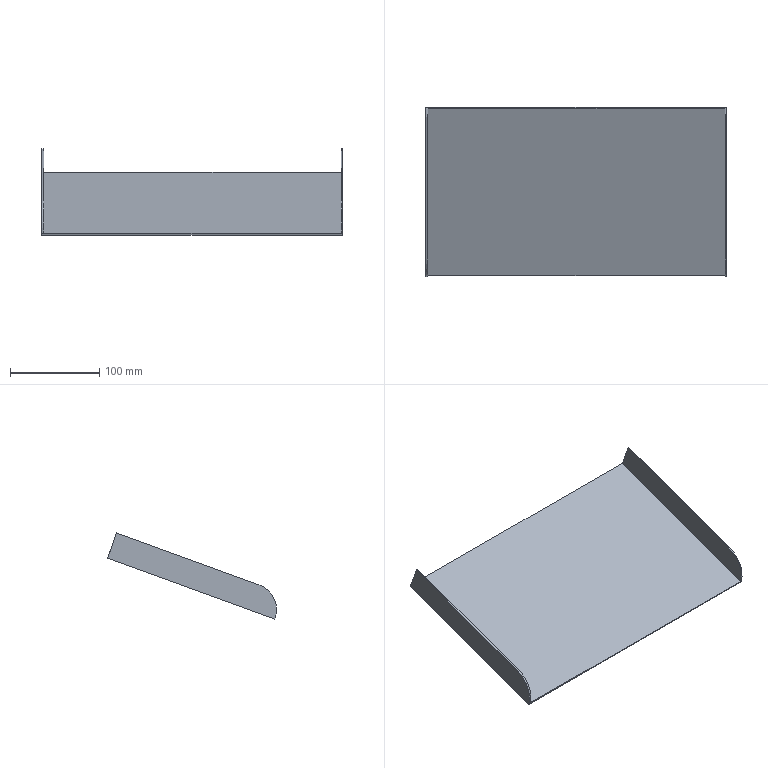Part | NX | features solid 2 | 1 solid | 12 faces | box 337.136 x 189.748 x 96.595 mm | volume 151075 mm3 | plane 10 | cylinder 2 | commonest cylinder face diameters 60 x2
STEP:
#1=CARTESIAN_POINT('',(-937.864,-997.876,-367.964));
#2=VERTEX_POINT('',#1);
#3=CARTESIAN_POINT('',(-938.864,-997.876,-367.964));
#4=VERTEX_POINT('',#3);
#5=CARTESIAN_POINT('',(-937.864,-997.876,-367.964));
#6=DIRECTION('',(1.,0.,0.));
#7=VECTOR('',#6,1000.);
#8=LINE('',#5,#7);
#9=EDGE_CURVE('',#2,#4,#8,.F.);
#10=ORIENTED_EDGE('',*,*,#9,.T.);
#11=CARTESIAN_POINT('',(-938.864,-810.,-299.582));
#12=VERTEX_POINT('',#11);
#13=CARTESIAN_POINT('',(-938.864,-838.191,-309.843));
#14=DIRECTION('',(0.,0.9397,0.342));
#15=VECTOR('',#14,1000.);
#16=LINE('',#13,#15);
#17=EDGE_CURVE('',#4,#12,#16,.T.);
#18=ORIENTED_EDGE('',*,*,#17,.T.);
#19=CARTESIAN_POINT('',(-1273.,-810.,-299.582));
#20=VERTEX_POINT('',#19);
#21=CARTESIAN_POINT('',(-1268.,-810.,-299.582));
#22=DIRECTION('',(-1.,0.,0.));
#23=VECTOR('',#22,1000.);
#24=LINE('',#21,#23);
#25=EDGE_CURVE('',#20,#12,#24,.F.);
#26=ORIENTED_EDGE('',*,*,#25,.F.);
#27=CARTESIAN_POINT('',(-1273.,-997.876,-367.964));
#28=VERTEX_POINT('',#27);
#29=CARTESIAN_POINT('',(-1273.,-838.191,-309.843));
#30=DIRECTION('',(0.,0.9397,0.342));
#31=VECTOR('',#30,1000.);
#32=LINE('',#29,#31);
#33=EDGE_CURVE('',#28,#20,#32,.T.);
#34=ORIENTED_EDGE('',*,*,#33,.F.);
#35=CARTESIAN_POINT('',(-1275.,-997.876,-367.964));
#36=VERTEX_POINT('',#35);
#37=CARTESIAN_POINT('',(-1280.,-997.876,-367.964));
#38=DIRECTION('',(-1.,0.,0.));
#39=VECTOR('',#38,1000.);
#40=LINE('',#37,#39);
#41=EDGE_CURVE('',#28,#36,#40,.T.);
#42=ORIENTED_EDGE('',*,*,#41,.T.);
#43=CARTESIAN_POINT('',(-1275.,-997.939,-367.986));
#44=VERTEX_POINT('',#43);
#45=CARTESIAN_POINT('',(-1275.,-838.191,-309.843));
#46=DIRECTION('',(0.,-0.9397,-0.342));
#47=VECTOR('',#46,1000.);
#48=LINE('',#45,#47);
#49=EDGE_CURVE('',#36,#44,#48,.T.);
#50=ORIENTED_EDGE('',*,*,#49,.T.);
#51=CARTESIAN_POINT('',(-937.864,-997.939,-367.986));
#52=VERTEX_POINT('',#51);
#53=CARTESIAN_POINT('',(-1268.,-997.939,-367.986));
#54=DIRECTION('',(1.,0.,0.));
#55=VECTOR('',#54,1000.);
#56=LINE('',#53,#55);
#57=EDGE_CURVE('',#44,#52,#56,.T.);
#58=ORIENTED_EDGE('',*,*,#57,.T.);
#59=CARTESIAN_POINT('',(-937.864,-838.191,-309.843));
#60=DIRECTION('',(0.,0.9397,0.342));
#61=VECTOR('',#60,1000.);
#62=LINE('',#59,#61);
#63=EDGE_CURVE('',#2,#52,#62,.F.);
#64=ORIENTED_EDGE('',*,*,#63,.F.);
#65=EDGE_LOOP('',(#10,#18,#26,#34,#42,#50,#58,#64));
#66=FACE_BOUND('',#65,.T.);
#67=CARTESIAN_POINT('',(-1268.,-838.191,-309.843));
#68=DIRECTION('',(0.,0.342,-0.9397));
#69=DIRECTION('',(-1.,0.,0.));
#70=AXIS2_PLACEMENT_3D('',#67,#68,#69);
#71=PLANE('',#70);
#72=ADVANCED_FACE('',(#66),#71,.F.);
#73=ORIENTED_EDGE('',*,*,#25,.T.);
#74=CARTESIAN_POINT('',(-938.864,-819.577,-273.271));
#75=VERTEX_POINT('',#74);
#76=CARTESIAN_POINT('',(-938.864,-809.316,-301.462));
#77=DIRECTION('',(0.,-0.342,0.9397));
#78=VECTOR('',#77,1000.);
#79=LINE('',#76,#78);
#80=EDGE_CURVE('',#12,#75,#79,.T.);
#81=ORIENTED_EDGE('',*,*,#80,.T.);
#82=CARTESIAN_POINT('',(-937.864,-819.577,-273.271));
#83=VERTEX_POINT('',#82);
#84=CARTESIAN_POINT('',(-937.864,-819.577,-273.271));
#85=DIRECTION('',(-1.,0.,0.));
#86=VECTOR('',#85,1000.);
#87=LINE('',#84,#86);
#88=EDGE_CURVE('',#83,#75,#87,.T.);
#89=ORIENTED_EDGE('',*,*,#88,.F.);
#90=CARTESIAN_POINT('',(-937.864,-809.316,-301.462));
#91=VERTEX_POINT('',#90);
#92=CARTESIAN_POINT('',(-937.864,-810.,-299.582));
#93=DIRECTION('',(0.,0.342,-0.9397));
#94=VECTOR('',#93,1000.);
#95=LINE('',#92,#94);
#96=EDGE_CURVE('',#83,#91,#95,.T.);
#97=ORIENTED_EDGE('',*,*,#96,.T.);
#98=CARTESIAN_POINT('',(-1275.,-809.316,-301.462));
#99=VERTEX_POINT('',#98);
#100=CARTESIAN_POINT('',(-1268.,-809.316,-301.462));
#101=DIRECTION('',(-1.,0.,0.));
#102=VECTOR('',#101,1000.);
#103=LINE('',#100,#102);
#104=EDGE_CURVE('',#99,#91,#103,.F.);
#105=ORIENTED_EDGE('',*,*,#104,.F.);
#106=CARTESIAN_POINT('',(-1275.,-819.577,-273.271));
#107=VERTEX_POINT('',#106);
#108=CARTESIAN_POINT('',(-1275.,-810.,-299.582));
#109=DIRECTION('',(0.,-0.342,0.9397));
#110=VECTOR('',#109,1000.);
#111=LINE('',#108,#110);
#112=EDGE_CURVE('',#107,#99,#111,.F.);
#113=ORIENTED_EDGE('',*,*,#112,.F.);
#114=CARTESIAN_POINT('',(-1273.,-819.577,-273.271));
#115=VERTEX_POINT('',#114);
#116=CARTESIAN_POINT('',(-1280.,-819.577,-273.271));
#117=DIRECTION('',(-1.,0.,0.));
#118=VECTOR('',#117,1000.);
#119=LINE('',#116,#118);
#120=EDGE_CURVE('',#107,#115,#119,.F.);
#121=ORIENTED_EDGE('',*,*,#120,.T.);
#122=CARTESIAN_POINT('',(-1273.,-809.316,-301.462));
#123=DIRECTION('',(0.,0.342,-0.9397));
#124=VECTOR('',#123,1000.);
#125=LINE('',#122,#124);
#126=EDGE_CURVE('',#20,#115,#125,.F.);
#127=ORIENTED_EDGE('',*,*,#126,.F.);
#128=EDGE_LOOP('',(#73,#81,#89,#97,#105,#113,#121,#127));
#129=FACE_BOUND('',#128,.T.);
#130=CARTESIAN_POINT('',(-1268.,-810.,-299.582));
#131=DIRECTION('',(0.,0.9397,0.342));
#132=DIRECTION('',(1.,0.,0.));
#133=AXIS2_PLACEMENT_3D('',#130,#131,#132);
#134=PLANE('',#133);
#135=ADVANCED_FACE('',(#129),#134,.T.);
#136=ORIENTED_EDGE('',*,*,#49,.F.);
#137=CARTESIAN_POINT('',(-1275.,-979.324,-331.414));
#138=VERTEX_POINT('',#137);
#139=CARTESIAN_POINT('',(-1275.,-969.064,-359.605));
#140=DIRECTION('',(1.,0.,0.));
#141=DIRECTION('',(0.,0.,-1.));
#142=AXIS2_PLACEMENT_3D('',#139,#140,#141);
#143=CIRCLE('',#142,30.);
#144=EDGE_CURVE('',#36,#138,#143,.F.);
#145=ORIENTED_EDGE('',*,*,#144,.T.);
#146=CARTESIAN_POINT('',(-1275.,-819.577,-273.271));
#147=DIRECTION('',(0.,-0.9397,-0.342));
#148=VECTOR('',#147,1000.);
#149=LINE('',#146,#148);
#150=EDGE_CURVE('',#107,#138,#149,.T.);
#151=ORIENTED_EDGE('',*,*,#150,.F.);
#152=ORIENTED_EDGE('',*,*,#112,.T.);
#153=CARTESIAN_POINT('',(-1275.,-997.254,-369.866));
#154=VERTEX_POINT('',#153);
#155=CARTESIAN_POINT('',(-1275.,-837.507,-311.722));
#156=DIRECTION('',(0.,-0.9397,-0.342));
#157=VECTOR('',#156,1000.);
#158=LINE('',#155,#157);
#159=EDGE_CURVE('',#99,#154,#158,.T.);
#160=ORIENTED_EDGE('',*,*,#159,.T.);
#161=CARTESIAN_POINT('',(-1275.,-997.939,-367.986));
#162=DIRECTION('',(0.,0.342,-0.9397));
#163=VECTOR('',#162,1000.);
#164=LINE('',#161,#163);
#165=EDGE_CURVE('',#44,#154,#164,.T.);
#166=ORIENTED_EDGE('',*,*,#165,.F.);
#167=EDGE_LOOP('',(#136,#145,#151,#152,#160,#166));
#168=FACE_BOUND('',#167,.T.);
#169=CARTESIAN_POINT('',(-1275.,-838.191,-309.843));
#170=DIRECTION('',(1.,0.,0.));
#171=DIRECTION('',(0.,-0.9397,-0.342));
#172=AXIS2_PLACEMENT_3D('',#169,#170,#171);
#173=PLANE('',#172);
#174=ADVANCED_FACE('',(#168),#173,.F.);
#175=ORIENTED_EDGE('',*,*,#165,.T.);
#176=CARTESIAN_POINT('',(-937.864,-997.254,-369.866));
#177=VERTEX_POINT('',#176);
#178=CARTESIAN_POINT('',(-1268.,-997.254,-369.866));
#179=DIRECTION('',(-1.,0.,0.));
#180=VECTOR('',#179,1000.);
#181=LINE('',#178,#180);
#182=EDGE_CURVE('',#154,#177,#181,.F.);
#183=ORIENTED_EDGE('',*,*,#182,.T.);
#184=CARTESIAN_POINT('',(-937.864,-997.939,-367.986));
#185=DIRECTION('',(0.,-0.342,0.9397));
#186=VECTOR('',#185,1000.);
#187=LINE('',#184,#186);
#188=EDGE_CURVE('',#52,#177,#187,.F.);
#189=ORIENTED_EDGE('',*,*,#188,.F.);
#190=ORIENTED_EDGE('',*,*,#57,.F.);
#191=EDGE_LOOP('',(#175,#183,#189,#190));
#192=FACE_BOUND('',#191,.T.);
#193=CARTESIAN_POINT('',(-1268.,-997.939,-367.986));
#194=DIRECTION('',(0.,0.9397,0.342));
#195=DIRECTION('',(1.,0.,0.));
#196=AXIS2_PLACEMENT_3D('',#193,#194,#195);
#197=PLANE('',#196);
#198=ADVANCED_FACE('',(#192),#197,.F.);
#199=ORIENTED_EDGE('',*,*,#188,.T.);
#200=CARTESIAN_POINT('',(-937.864,-837.507,-311.722));
#201=DIRECTION('',(0.,0.9397,0.342));
#202=VECTOR('',#201,1000.);
#203=LINE('',#200,#202);
#204=EDGE_CURVE('',#91,#177,#203,.F.);
#205=ORIENTED_EDGE('',*,*,#204,.F.);
#206=ORIENTED_EDGE('',*,*,#96,.F.);
#207=CARTESIAN_POINT('',(-937.864,-979.324,-331.414));
#208=VERTEX_POINT('',#207);
#209=CARTESIAN_POINT('',(-937.864,-819.577,-273.271));
#210=DIRECTION('',(0.,-0.9397,-0.342));
#211=VECTOR('',#210,1000.);
#212=LINE('',#209,#211);
#213=EDGE_CURVE('',#83,#208,#212,.T.);
#214=ORIENTED_EDGE('',*,*,#213,.T.);
#215=CARTESIAN_POINT('',(-937.864,-969.064,-359.605));
#216=DIRECTION('',(-1.,0.,0.));
#217=DIRECTION('',(0.,-0.342,0.9397));
#218=AXIS2_PLACEMENT_3D('',#215,#216,#217);
#219=CIRCLE('',#218,30.);
#220=EDGE_CURVE('',#208,#2,#219,.F.);
#221=ORIENTED_EDGE('',*,*,#220,.T.);
#222=ORIENTED_EDGE('',*,*,#63,.T.);
#223=EDGE_LOOP('',(#199,#205,#206,#214,#221,#222));
#224=FACE_BOUND('',#223,.T.);
#225=CARTESIAN_POINT('',(-937.864,-838.191,-309.843));
#226=DIRECTION('',(1.,0.,0.));
#227=DIRECTION('',(0.,-0.9397,-0.342));
#228=AXIS2_PLACEMENT_3D('',#225,#226,#227);
#229=PLANE('',#228);
#230=ADVANCED_FACE('',(#224),#229,.T.);
#231=ORIENTED_EDGE('',*,*,#104,.T.);
#232=ORIENTED_EDGE('',*,*,#204,.T.);
#233=ORIENTED_EDGE('',*,*,#182,.F.);
#234=ORIENTED_EDGE('',*,*,#159,.F.);
#235=EDGE_LOOP('',(#231,#232,#233,#234));
#236=FACE_BOUND('',#235,.T.);
#237=CARTESIAN_POINT('',(-1268.,-837.507,-311.722));
#238=DIRECTION('',(0.,0.342,-0.9397));
#239=DIRECTION('',(-1.,0.,0.));
#240=AXIS2_PLACEMENT_3D('',#237,#238,#239);
#241=PLANE('',#240);
#242=ADVANCED_FACE('',(#236),#241,.T.);
#243=CARTESIAN_POINT('',(-1273.,-979.324,-331.414));
#244=VERTEX_POINT('',#243);
#245=CARTESIAN_POINT('',(-1273.,-969.064,-359.605));
#246=DIRECTION('',(-1.,0.,0.));
#247=DIRECTION('',(0.,0.,1.));
#248=AXIS2_PLACEMENT_3D('',#245,#246,#247);
#249=CIRCLE('',#248,30.);
#250=EDGE_CURVE('',#244,#28,#249,.F.);
#251=ORIENTED_EDGE('',*,*,#250,.T.);
#252=ORIENTED_EDGE('',*,*,#33,.T.);
#253=ORIENTED_EDGE('',*,*,#126,.T.);
#254=CARTESIAN_POINT('',(-1273.,-819.577,-273.271));
#255=DIRECTION('',(0.,-0.9397,-0.342));
#256=VECTOR('',#255,1000.);
#257=LINE('',#254,#256);
#258=EDGE_CURVE('',#115,#244,#257,.T.);
#259=ORIENTED_EDGE('',*,*,#258,.T.);
#260=EDGE_LOOP('',(#251,#252,#253,#259));
#261=FACE_BOUND('',#260,.T.);
#262=CARTESIAN_POINT('',(-1273.,-809.316,-301.462));
#263=DIRECTION('',(-1.,0.,0.));
#264=DIRECTION('',(0.,-0.342,0.9397));
#265=AXIS2_PLACEMENT_3D('',#262,#263,#264);
#266=PLANE('',#265);
#267=ADVANCED_FACE('',(#261),#266,.F.);
#268=ORIENTED_EDGE('',*,*,#41,.F.);
#269=ORIENTED_EDGE('',*,*,#250,.F.);
#270=CARTESIAN_POINT('',(-1280.,-979.324,-331.414));
#271=DIRECTION('',(-1.,0.,0.));
#272=VECTOR('',#271,1000.);
#273=LINE('',#270,#272);
#274=EDGE_CURVE('',#138,#244,#273,.F.);
#275=ORIENTED_EDGE('',*,*,#274,.F.);
#276=ORIENTED_EDGE('',*,*,#144,.F.);
#277=EDGE_LOOP('',(#268,#269,#275,#276));
#278=FACE_BOUND('',#277,.T.);
#279=CARTESIAN_POINT('',(-1280.,-969.064,-359.605));
#280=DIRECTION('',(-1.,0.,0.));
#281=DIRECTION('',(0.,-0.342,0.9397));
#282=AXIS2_PLACEMENT_3D('',#279,#280,#281);
#283=CYLINDRICAL_SURFACE('',#282,30.);
#284=ADVANCED_FACE('',(#278),#283,.T.);
#285=ORIENTED_EDGE('',*,*,#150,.T.);
#286=ORIENTED_EDGE('',*,*,#274,.T.);
#287=ORIENTED_EDGE('',*,*,#258,.F.);
#288=ORIENTED_EDGE('',*,*,#120,.F.);
#289=EDGE_LOOP('',(#285,#286,#287,#288));
#290=FACE_BOUND('',#289,.T.);
#291=CARTESIAN_POINT('',(-1280.,-819.577,-273.271));
#292=DIRECTION('',(0.,0.342,-0.9397));
#293=DIRECTION('',(0.,-0.9397,-0.342));
#294=AXIS2_PLACEMENT_3D('',#291,#292,#293);
#295=PLANE('',#294);
#296=ADVANCED_FACE('',(#290),#295,.F.);
#297=ORIENTED_EDGE('',*,*,#17,.F.);
#298=CARTESIAN_POINT('',(-938.864,-979.324,-331.414));
#299=VERTEX_POINT('',#298);
#300=CARTESIAN_POINT('',(-938.864,-969.064,-359.605));
#301=DIRECTION('',(-1.,0.,0.));
#302=DIRECTION('',(0.,-0.342,0.9397));
#303=AXIS2_PLACEMENT_3D('',#300,#301,#302);
#304=CIRCLE('',#303,30.);
#305=EDGE_CURVE('',#4,#299,#304,.T.);
#306=ORIENTED_EDGE('',*,*,#305,.T.);
#307=CARTESIAN_POINT('',(-938.864,-819.577,-273.271));
#308=DIRECTION('',(0.,0.9397,0.342));
#309=VECTOR('',#308,1000.);
#310=LINE('',#307,#309);
#311=EDGE_CURVE('',#75,#299,#310,.F.);
#312=ORIENTED_EDGE('',*,*,#311,.F.);
#313=ORIENTED_EDGE('',*,*,#80,.F.);
#314=EDGE_LOOP('',(#297,#306,#312,#313));
#315=FACE_BOUND('',#314,.T.);
#316=CARTESIAN_POINT('',(-938.864,-809.316,-301.462));
#317=DIRECTION('',(-1.,0.,0.));
#318=DIRECTION('',(0.,-0.342,0.9397));
#319=AXIS2_PLACEMENT_3D('',#316,#317,#318);
#320=PLANE('',#319);
#321=ADVANCED_FACE('',(#315),#320,.T.);
#322=ORIENTED_EDGE('',*,*,#9,.F.);
#323=ORIENTED_EDGE('',*,*,#220,.F.);
#324=CARTESIAN_POINT('',(-937.864,-979.324,-331.414));
#325=DIRECTION('',(-1.,0.,0.));
#326=VECTOR('',#325,1000.);
#327=LINE('',#324,#326);
#328=EDGE_CURVE('',#299,#208,#327,.F.);
#329=ORIENTED_EDGE('',*,*,#328,.F.);
#330=ORIENTED_EDGE('',*,*,#305,.F.);
#331=EDGE_LOOP('',(#322,#323,#329,#330));
#332=FACE_BOUND('',#331,.T.);
#333=CARTESIAN_POINT('',(-937.864,-969.064,-359.605));
#334=DIRECTION('',(1.,0.,0.));
#335=DIRECTION('',(0.,0.342,-0.9397));
#336=AXIS2_PLACEMENT_3D('',#333,#334,#335);
#337=CYLINDRICAL_SURFACE('',#336,30.);
#338=ADVANCED_FACE('',(#332),#337,.T.);
#339=ORIENTED_EDGE('',*,*,#311,.T.);
#340=ORIENTED_EDGE('',*,*,#328,.T.);
#341=ORIENTED_EDGE('',*,*,#213,.F.);
#342=ORIENTED_EDGE('',*,*,#88,.T.);
#343=EDGE_LOOP('',(#339,#340,#341,#342));
#344=FACE_BOUND('',#343,.T.);
#345=CARTESIAN_POINT('',(-937.864,-819.577,-273.271));
#346=DIRECTION('',(0.,0.342,-0.9397));
#347=DIRECTION('',(0.,-0.9397,-0.342));
#348=AXIS2_PLACEMENT_3D('',#345,#346,#347);
#349=PLANE('',#348);
#350=ADVANCED_FACE('',(#344),#349,.F.);
#351=CLOSED_SHELL('',(#72,#135,#174,#198,#230,#242,#267,#284,#296,#321,#338,#350));
#352=MANIFOLD_SOLID_BREP('',#351);
#353=(LENGTH_UNIT()NAMED_UNIT(*)SI_UNIT(.MILLI.,.METRE.));
#354=UNCERTAINTY_MEASURE_WITH_UNIT(LENGTH_MEASURE(0.00001),#353,'','');
#355=(NAMED_UNIT(*)PLANE_ANGLE_UNIT()SI_UNIT($,.RADIAN.));
#356=(NAMED_UNIT(*)SI_UNIT($,.STERADIAN.)SOLID_ANGLE_UNIT());
#357=(GEOMETRIC_REPRESENTATION_CONTEXT(3)GLOBAL_UNCERTAINTY_ASSIGNED_CONTEXT((#354))GLOBAL_UNIT_ASSIGNED_CONTEXT((#353,#355,#356))REPRESENTATION_CONTEXT('',''));
#358=ADVANCED_BREP_SHAPE_REPRESENTATION('',(#352),#357);